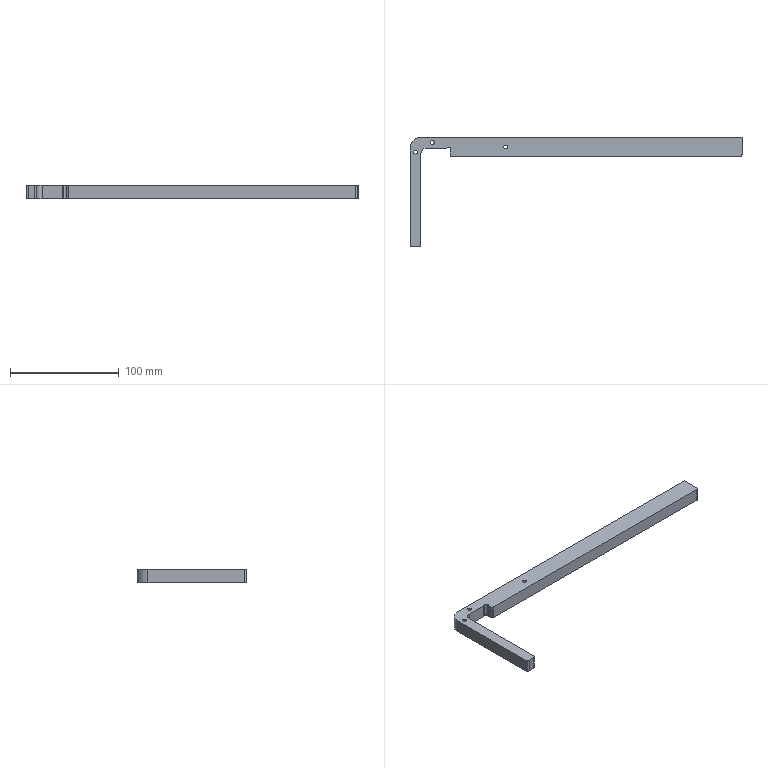Part | STEP file | ASND-0110-PWP TOP tu pang 20130814.sldasm-Part-8aq | 1 solid | 40 faces | box 305.546 x 101 x 12 mm | volume 72445 mm3 | cylinder 27 | plane 13 | commonest cylinder face diameters 4 x13 3.5 x6 6 x6 10 x1 20 x1